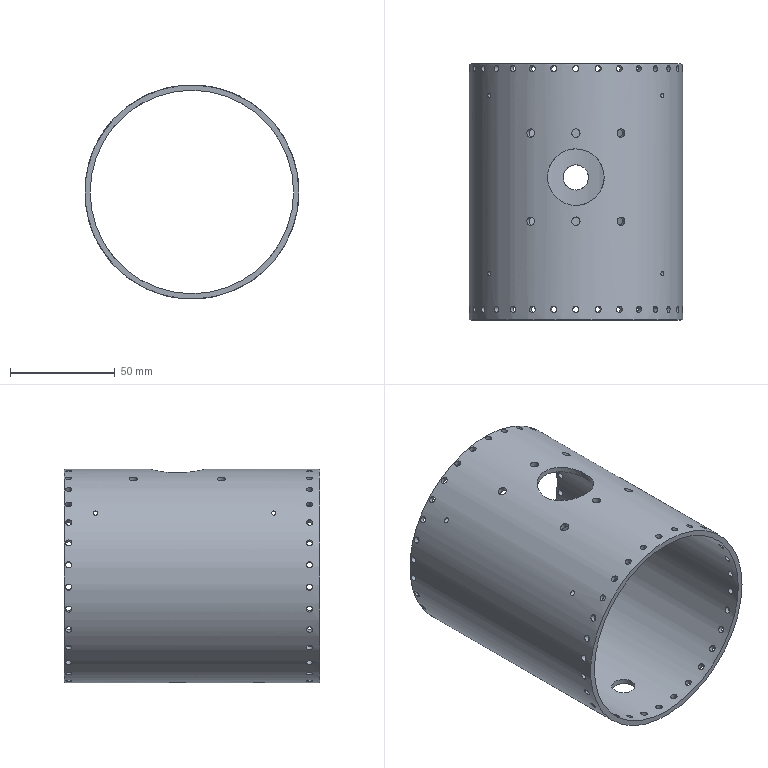Part | STEP file | 1-56.2 | 1 solid | 78 faces | box 102 x 122 x 102 mm | volume 92054 mm3 | cylinder 76 | plane 2 | commonest cylinder face diameters 3 x60 4 x7 2 x4 11 x1 12 x1 27 x1